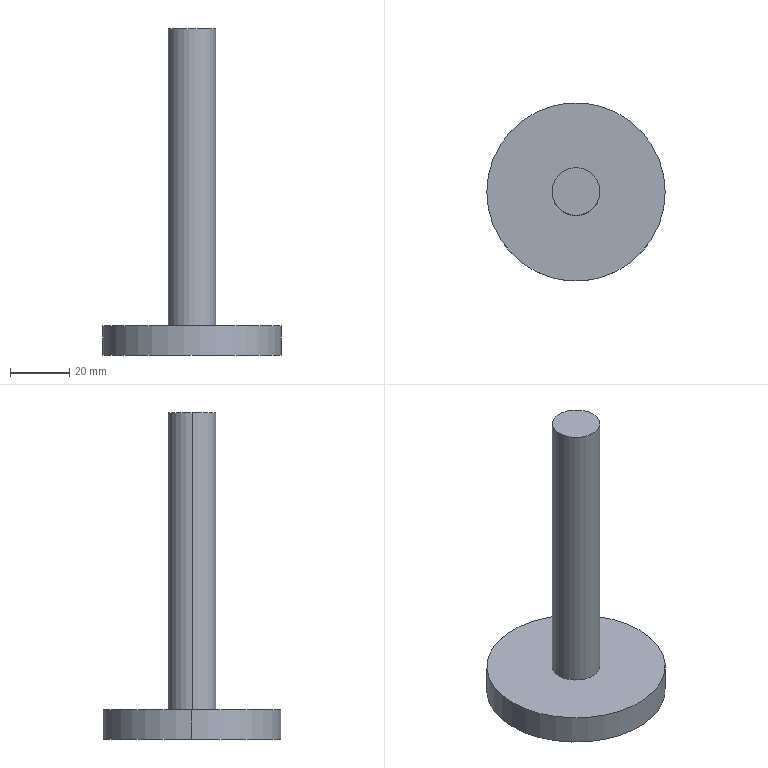Part | STEP file | CHAN TANGDUA | 1 solid | 7 faces | box 60 x 60 x 110 mm | volume 48381 mm3 | cylinder 4 | plane 3 | commonest cylinder face diameters 16 x2 60 x2
STEP:
#1=CARTESIAN_POINT('',(0.,0.,0.));
#2=DIRECTION('',(0.,0.,1.));
#3=DIRECTION('',(1.,0.,0.));
#4=AXIS2_PLACEMENT_3D('',#1,#2,#3);
#5=CARTESIAN_POINT('',(8.,0.,10.));
#6=VERTEX_POINT('',#5);
#7=CARTESIAN_POINT('',(-8.,0.,10.));
#8=VERTEX_POINT('',#7);
#9=CARTESIAN_POINT('',(0.,0.,10.));
#10=DIRECTION('',(0.,0.,1.));
#11=DIRECTION('',(1.,0.,0.));
#12=AXIS2_PLACEMENT_3D('',#9,#10,#11);
#13=CIRCLE('',#12,8.);
#14=CARTESIAN_POINT('',(0.,0.,10.));
#15=DIRECTION('',(0.,0.,1.));
#16=DIRECTION('',(1.,0.,0.));
#17=AXIS2_PLACEMENT_3D('',#14,#15,#16);
#18=CYLINDRICAL_SURFACE('',#17,8.);
#19=CARTESIAN_POINT('',(0.,0.));
#20=DIRECTION('',(1.,0.));
#21=VECTOR('',#20,1.);
#22=LINE('',#19,#21);
#23=(GEOMETRIC_REPRESENTATION_CONTEXT(2)PARAMETRIC_REPRESENTATION_CONTEXT()REPRESENTATION_CONTEXT('',''));
#24=DEFINITIONAL_REPRESENTATION('',(#22),#23);
#25=PCURVE('',#18,#24);
#26=CARTESIAN_POINT('',(0.,0.,10.));
#27=DIRECTION('',(0.,0.,-1.));
#28=DIRECTION('',(-1.,0.,0.));
#29=AXIS2_PLACEMENT_3D('',#26,#27,#28);
#30=PLANE('',#29);
#31=CARTESIAN_POINT('',(-8.,0.));
#32=CARTESIAN_POINT('',(-8.,13.856));
#33=CARTESIAN_POINT('',(4.,6.928));
#34=CARTESIAN_POINT('',(16.,0.));
#35=CARTESIAN_POINT('',(4.,-6.928));
#36=CARTESIAN_POINT('',(-8.,-13.856));
#37=CARTESIAN_POINT('',(-8.,0.));
#38=(BOUNDED_CURVE()B_SPLINE_CURVE(2,(#31,#32,#33,#34,#35,#36,#37),.UNSPECIFIED.,.T.,.F.)B_SPLINE_CURVE_WITH_KNOTS((1,2,2,2,2,1),(-2.094,0.,2.094,4.189,6.283,8.378),.UNSPECIFIED.)CURVE()GEOMETRIC_REPRESENTATION_ITEM()RATIONAL_B_SPLINE_CURVE((1.,0.5,1.,0.5,1.,0.5,1.))REPRESENTATION_ITEM(''));
#39=(GEOMETRIC_REPRESENTATION_CONTEXT(2)PARAMETRIC_REPRESENTATION_CONTEXT()REPRESENTATION_CONTEXT('',''));
#40=DEFINITIONAL_REPRESENTATION('',(#38),#39);
#41=PCURVE('',#30,#40);
#42=SURFACE_CURVE('',#13,(#25,#41),.PCURVE_S1.);
#43=EDGE_CURVE('',#6,#8,#42,.T.);
#44=ORIENTED_EDGE('',*,*,#43,.T.);
#45=CARTESIAN_POINT('',(-8.,0.,110.));
#46=VERTEX_POINT('',#45);
#47=CARTESIAN_POINT('',(-8.,0.,10.));
#48=DIRECTION('',(0.,0.,1.));
#49=VECTOR('',#48,1.);
#50=LINE('',#47,#49);
#51=CARTESIAN_POINT('',(3.142,0.));
#52=DIRECTION('',(0.,1.));
#53=VECTOR('',#52,1.);
#54=LINE('',#51,#53);
#55=(GEOMETRIC_REPRESENTATION_CONTEXT(2)PARAMETRIC_REPRESENTATION_CONTEXT()REPRESENTATION_CONTEXT('',''));
#56=DEFINITIONAL_REPRESENTATION('',(#54),#55);
#57=PCURVE('',#18,#56);
#58=CARTESIAN_POINT('',(0.,0.,10.));
#59=DIRECTION('',(0.,0.,1.));
#60=DIRECTION('',(1.,0.,0.));
#61=AXIS2_PLACEMENT_3D('',#58,#59,#60);
#62=CYLINDRICAL_SURFACE('',#61,8.);
#63=CARTESIAN_POINT('',(3.142,0.));
#64=DIRECTION('',(0.,1.));
#65=VECTOR('',#64,1.);
#66=LINE('',#63,#65);
#67=(GEOMETRIC_REPRESENTATION_CONTEXT(2)PARAMETRIC_REPRESENTATION_CONTEXT()REPRESENTATION_CONTEXT('',''));
#68=DEFINITIONAL_REPRESENTATION('',(#66),#67);
#69=PCURVE('',#62,#68);
#70=SURFACE_CURVE('',#50,(#57,#69),.PCURVE_S1.);
#71=EDGE_CURVE('',#8,#46,#70,.T.);
#72=ORIENTED_EDGE('',*,*,#71,.T.);
#73=CARTESIAN_POINT('',(8.,0.,110.));
#74=VERTEX_POINT('',#73);
#75=CARTESIAN_POINT('',(0.,0.,110.));
#76=DIRECTION('',(0.,0.,-1.));
#77=DIRECTION('',(1.,0.,0.));
#78=AXIS2_PLACEMENT_3D('',#75,#76,#77);
#79=CIRCLE('',#78,8.);
#80=CARTESIAN_POINT('',(6.283,100.));
#81=DIRECTION('',(-1.,0.));
#82=VECTOR('',#81,1.);
#83=LINE('',#80,#82);
#84=(GEOMETRIC_REPRESENTATION_CONTEXT(2)PARAMETRIC_REPRESENTATION_CONTEXT()REPRESENTATION_CONTEXT('',''));
#85=DEFINITIONAL_REPRESENTATION('',(#83),#84);
#86=PCURVE('',#18,#85);
#87=CARTESIAN_POINT('',(0.,0.,110.));
#88=DIRECTION('',(0.,0.,-1.));
#89=DIRECTION('',(-1.,0.,0.));
#90=AXIS2_PLACEMENT_3D('',#87,#88,#89);
#91=PLANE('',#90);
#92=CARTESIAN_POINT('',(0.,0.));
#93=DIRECTION('',(-1.,0.));
#94=AXIS2_PLACEMENT_2D('',#92,#93);
#95=CIRCLE('',#94,8.);
#96=(GEOMETRIC_REPRESENTATION_CONTEXT(2)PARAMETRIC_REPRESENTATION_CONTEXT()REPRESENTATION_CONTEXT('',''));
#97=DEFINITIONAL_REPRESENTATION('',(#95),#96);
#98=PCURVE('',#91,#97);
#99=SURFACE_CURVE('',#79,(#86,#98),.PCURVE_S1.);
#100=EDGE_CURVE('',#46,#74,#99,.T.);
#101=ORIENTED_EDGE('',*,*,#100,.T.);
#102=CARTESIAN_POINT('',(8.,0.,10.));
#103=DIRECTION('',(0.,0.,1.));
#104=VECTOR('',#103,1.);
#105=LINE('',#102,#104);
#106=CARTESIAN_POINT('',(0.,0.));
#107=DIRECTION('',(0.,1.));
#108=VECTOR('',#107,1.);
#109=LINE('',#106,#108);
#110=(GEOMETRIC_REPRESENTATION_CONTEXT(2)PARAMETRIC_REPRESENTATION_CONTEXT()REPRESENTATION_CONTEXT('',''));
#111=DEFINITIONAL_REPRESENTATION('',(#109),#110);
#112=PCURVE('',#18,#111);
#113=CARTESIAN_POINT('',(6.283,0.));
#114=DIRECTION('',(0.,1.));
#115=VECTOR('',#114,1.);
#116=LINE('',#113,#115);
#117=(GEOMETRIC_REPRESENTATION_CONTEXT(2)PARAMETRIC_REPRESENTATION_CONTEXT()REPRESENTATION_CONTEXT('',''));
#118=DEFINITIONAL_REPRESENTATION('',(#116),#117);
#119=PCURVE('',#62,#118);
#120=SURFACE_CURVE('',#105,(#112,#119),.PCURVE_S1.);
#121=EDGE_CURVE('',#6,#74,#120,.T.);
#122=ORIENTED_EDGE('',*,*,#121,.F.);
#123=EDGE_LOOP('',(#44,#72,#101,#122));
#124=FACE_BOUND('',#123,.T.);
#125=ADVANCED_FACE('',(#124),#18,.T.);
#126=CARTESIAN_POINT('',(30.,0.,0.));
#127=VERTEX_POINT('',#126);
#128=CARTESIAN_POINT('',(-30.,0.,0.));
#129=VERTEX_POINT('',#128);
#130=CARTESIAN_POINT('',(0.,0.,0.));
#131=DIRECTION('',(0.,0.,1.));
#132=DIRECTION('',(1.,0.,0.));
#133=AXIS2_PLACEMENT_3D('',#130,#131,#132);
#134=CIRCLE('',#133,30.);
#135=CARTESIAN_POINT('',(0.,0.,0.));
#136=DIRECTION('',(0.,0.,1.));
#137=DIRECTION('',(1.,0.,0.));
#138=AXIS2_PLACEMENT_3D('',#135,#136,#137);
#139=CYLINDRICAL_SURFACE('',#138,30.);
#140=CARTESIAN_POINT('',(0.,0.));
#141=DIRECTION('',(1.,0.));
#142=VECTOR('',#141,1.);
#143=LINE('',#140,#142);
#144=(GEOMETRIC_REPRESENTATION_CONTEXT(2)PARAMETRIC_REPRESENTATION_CONTEXT()REPRESENTATION_CONTEXT('',''));
#145=DEFINITIONAL_REPRESENTATION('',(#143),#144);
#146=PCURVE('',#139,#145);
#147=CARTESIAN_POINT('',(0.,0.,0.));
#148=DIRECTION('',(0.,0.,-1.));
#149=DIRECTION('',(-1.,0.,0.));
#150=AXIS2_PLACEMENT_3D('',#147,#148,#149);
#151=PLANE('',#150);
#152=CARTESIAN_POINT('',(-30.,0.));
#153=CARTESIAN_POINT('',(-30.,51.962));
#154=CARTESIAN_POINT('',(15.,25.981));
#155=CARTESIAN_POINT('',(60.,0.));
#156=CARTESIAN_POINT('',(15.,-25.981));
#157=CARTESIAN_POINT('',(-30.,-51.962));
#158=CARTESIAN_POINT('',(-30.,0.));
#159=(BOUNDED_CURVE()B_SPLINE_CURVE(2,(#152,#153,#154,#155,#156,#157,#158),.UNSPECIFIED.,.T.,.F.)B_SPLINE_CURVE_WITH_KNOTS((1,2,2,2,2,1),(-2.094,0.,2.094,4.189,6.283,8.378),.UNSPECIFIED.)CURVE()GEOMETRIC_REPRESENTATION_ITEM()RATIONAL_B_SPLINE_CURVE((1.,0.5,1.,0.5,1.,0.5,1.))REPRESENTATION_ITEM(''));
#160=(GEOMETRIC_REPRESENTATION_CONTEXT(2)PARAMETRIC_REPRESENTATION_CONTEXT()REPRESENTATION_CONTEXT('',''));
#161=DEFINITIONAL_REPRESENTATION('',(#159),#160);
#162=PCURVE('',#151,#161);
#163=SURFACE_CURVE('',#134,(#146,#162),.PCURVE_S1.);
#164=EDGE_CURVE('',#127,#129,#163,.T.);
#165=ORIENTED_EDGE('',*,*,#164,.T.);
#166=CARTESIAN_POINT('',(-30.,0.,10.));
#167=VERTEX_POINT('',#166);
#168=CARTESIAN_POINT('',(-30.,0.,0.));
#169=DIRECTION('',(0.,0.,1.));
#170=VECTOR('',#169,1.);
#171=LINE('',#168,#170);
#172=CARTESIAN_POINT('',(3.142,0.));
#173=DIRECTION('',(0.,1.));
#174=VECTOR('',#173,1.);
#175=LINE('',#172,#174);
#176=(GEOMETRIC_REPRESENTATION_CONTEXT(2)PARAMETRIC_REPRESENTATION_CONTEXT()REPRESENTATION_CONTEXT('',''));
#177=DEFINITIONAL_REPRESENTATION('',(#175),#176);
#178=PCURVE('',#139,#177);
#179=CARTESIAN_POINT('',(0.,0.,0.));
#180=DIRECTION('',(0.,0.,1.));
#181=DIRECTION('',(1.,0.,0.));
#182=AXIS2_PLACEMENT_3D('',#179,#180,#181);
#183=CYLINDRICAL_SURFACE('',#182,30.);
#184=CARTESIAN_POINT('',(3.142,0.));
#185=DIRECTION('',(0.,1.));
#186=VECTOR('',#185,1.);
#187=LINE('',#184,#186);
#188=(GEOMETRIC_REPRESENTATION_CONTEXT(2)PARAMETRIC_REPRESENTATION_CONTEXT()REPRESENTATION_CONTEXT('',''));
#189=DEFINITIONAL_REPRESENTATION('',(#187),#188);
#190=PCURVE('',#183,#189);
#191=SURFACE_CURVE('',#171,(#178,#190),.PCURVE_S1.);
#192=EDGE_CURVE('',#129,#167,#191,.T.);
#193=ORIENTED_EDGE('',*,*,#192,.T.);
#194=CARTESIAN_POINT('',(30.,0.,10.));
#195=VERTEX_POINT('',#194);
#196=CARTESIAN_POINT('',(0.,0.,10.));
#197=DIRECTION('',(0.,0.,-1.));
#198=DIRECTION('',(1.,0.,0.));
#199=AXIS2_PLACEMENT_3D('',#196,#197,#198);
#200=CIRCLE('',#199,30.);
#201=CARTESIAN_POINT('',(6.283,10.));
#202=DIRECTION('',(-1.,0.));
#203=VECTOR('',#202,1.);
#204=LINE('',#201,#203);
#205=(GEOMETRIC_REPRESENTATION_CONTEXT(2)PARAMETRIC_REPRESENTATION_CONTEXT()REPRESENTATION_CONTEXT('',''));
#206=DEFINITIONAL_REPRESENTATION('',(#204),#205);
#207=PCURVE('',#139,#206);
#208=CARTESIAN_POINT('',(0.,0.));
#209=DIRECTION('',(-1.,0.));
#210=AXIS2_PLACEMENT_2D('',#208,#209);
#211=CIRCLE('',#210,30.);
#212=(GEOMETRIC_REPRESENTATION_CONTEXT(2)PARAMETRIC_REPRESENTATION_CONTEXT()REPRESENTATION_CONTEXT('',''));
#213=DEFINITIONAL_REPRESENTATION('',(#211),#212);
#214=PCURVE('',#30,#213);
#215=SURFACE_CURVE('',#200,(#207,#214),.PCURVE_S1.);
#216=EDGE_CURVE('',#167,#195,#215,.T.);
#217=ORIENTED_EDGE('',*,*,#216,.T.);
#218=CARTESIAN_POINT('',(30.,0.,0.));
#219=DIRECTION('',(0.,0.,1.));
#220=VECTOR('',#219,1.);
#221=LINE('',#218,#220);
#222=CARTESIAN_POINT('',(0.,0.));
#223=DIRECTION('',(0.,1.));
#224=VECTOR('',#223,1.);
#225=LINE('',#222,#224);
#226=(GEOMETRIC_REPRESENTATION_CONTEXT(2)PARAMETRIC_REPRESENTATION_CONTEXT()REPRESENTATION_CONTEXT('',''));
#227=DEFINITIONAL_REPRESENTATION('',(#225),#226);
#228=PCURVE('',#139,#227);
#229=CARTESIAN_POINT('',(6.283,0.));
#230=DIRECTION('',(0.,1.));
#231=VECTOR('',#230,1.);
#232=LINE('',#229,#231);
#233=(GEOMETRIC_REPRESENTATION_CONTEXT(2)PARAMETRIC_REPRESENTATION_CONTEXT()REPRESENTATION_CONTEXT('',''));
#234=DEFINITIONAL_REPRESENTATION('',(#232),#233);
#235=PCURVE('',#183,#234);
#236=SURFACE_CURVE('',#221,(#228,#235),.PCURVE_S1.);
#237=EDGE_CURVE('',#127,#195,#236,.T.);
#238=ORIENTED_EDGE('',*,*,#237,.F.);
#239=EDGE_LOOP('',(#165,#193,#217,#238));
#240=FACE_BOUND('',#239,.T.);
#241=ADVANCED_FACE('',(#240),#139,.T.);
#242=ORIENTED_EDGE('',*,*,#71,.F.);
#243=CARTESIAN_POINT('',(0.,0.,10.));
#244=DIRECTION('',(0.,0.,1.));
#245=DIRECTION('',(1.,0.,0.));
#246=AXIS2_PLACEMENT_3D('',#243,#244,#245);
#247=CIRCLE('',#246,8.);
#248=CARTESIAN_POINT('',(0.,0.));
#249=DIRECTION('',(1.,0.));
#250=VECTOR('',#249,1.);
#251=LINE('',#248,#250);
#252=(GEOMETRIC_REPRESENTATION_CONTEXT(2)PARAMETRIC_REPRESENTATION_CONTEXT()REPRESENTATION_CONTEXT('',''));
#253=DEFINITIONAL_REPRESENTATION('',(#251),#252);
#254=PCURVE('',#62,#253);
#255=CARTESIAN_POINT('',(-8.,0.));
#256=CARTESIAN_POINT('',(-8.,13.856));
#257=CARTESIAN_POINT('',(4.,6.928));
#258=CARTESIAN_POINT('',(16.,0.));
#259=CARTESIAN_POINT('',(4.,-6.928));
#260=CARTESIAN_POINT('',(-8.,-13.856));
#261=CARTESIAN_POINT('',(-8.,0.));
#262=(BOUNDED_CURVE()B_SPLINE_CURVE(2,(#255,#256,#257,#258,#259,#260,#261),.UNSPECIFIED.,.T.,.F.)B_SPLINE_CURVE_WITH_KNOTS((1,2,2,2,2,1),(-2.094,0.,2.094,4.189,6.283,8.378),.UNSPECIFIED.)CURVE()GEOMETRIC_REPRESENTATION_ITEM()RATIONAL_B_SPLINE_CURVE((1.,0.5,1.,0.5,1.,0.5,1.))REPRESENTATION_ITEM(''));
#263=(GEOMETRIC_REPRESENTATION_CONTEXT(2)PARAMETRIC_REPRESENTATION_CONTEXT()REPRESENTATION_CONTEXT('',''));
#264=DEFINITIONAL_REPRESENTATION('',(#262),#263);
#265=PCURVE('',#30,#264);
#266=SURFACE_CURVE('',#247,(#254,#265),.PCURVE_S1.);
#267=EDGE_CURVE('',#8,#6,#266,.T.);
#268=ORIENTED_EDGE('',*,*,#267,.T.);
#269=ORIENTED_EDGE('',*,*,#121,.T.);
#270=CARTESIAN_POINT('',(0.,0.,110.));
#271=DIRECTION('',(0.,0.,-1.));
#272=DIRECTION('',(1.,0.,0.));
#273=AXIS2_PLACEMENT_3D('',#270,#271,#272);
#274=CIRCLE('',#273,8.);
#275=CARTESIAN_POINT('',(6.283,100.));
#276=DIRECTION('',(-1.,0.));
#277=VECTOR('',#276,1.);
#278=LINE('',#275,#277);
#279=(GEOMETRIC_REPRESENTATION_CONTEXT(2)PARAMETRIC_REPRESENTATION_CONTEXT()REPRESENTATION_CONTEXT('',''));
#280=DEFINITIONAL_REPRESENTATION('',(#278),#279);
#281=PCURVE('',#62,#280);
#282=CARTESIAN_POINT('',(0.,0.));
#283=DIRECTION('',(-1.,0.));
#284=AXIS2_PLACEMENT_2D('',#282,#283);
#285=CIRCLE('',#284,8.);
#286=(GEOMETRIC_REPRESENTATION_CONTEXT(2)PARAMETRIC_REPRESENTATION_CONTEXT()REPRESENTATION_CONTEXT('',''));
#287=DEFINITIONAL_REPRESENTATION('',(#285),#286);
#288=PCURVE('',#91,#287);
#289=SURFACE_CURVE('',#274,(#281,#288),.PCURVE_S1.);
#290=EDGE_CURVE('',#74,#46,#289,.T.);
#291=ORIENTED_EDGE('',*,*,#290,.T.);
#292=EDGE_LOOP('',(#242,#268,#269,#291));
#293=FACE_BOUND('',#292,.T.);
#294=ADVANCED_FACE('',(#293),#62,.T.);
#295=ORIENTED_EDGE('',*,*,#43,.F.);
#296=ORIENTED_EDGE('',*,*,#267,.F.);
#297=EDGE_LOOP('',(#295,#296));
#298=FACE_BOUND('',#297,.T.);
#299=CARTESIAN_POINT('',(0.,0.,10.));
#300=DIRECTION('',(0.,0.,-1.));
#301=DIRECTION('',(1.,0.,0.));
#302=AXIS2_PLACEMENT_3D('',#299,#300,#301);
#303=CIRCLE('',#302,30.);
#304=CARTESIAN_POINT('',(0.,0.));
#305=DIRECTION('',(-1.,0.));
#306=AXIS2_PLACEMENT_2D('',#304,#305);
#307=CIRCLE('',#306,30.);
#308=(GEOMETRIC_REPRESENTATION_CONTEXT(2)PARAMETRIC_REPRESENTATION_CONTEXT()REPRESENTATION_CONTEXT('',''));
#309=DEFINITIONAL_REPRESENTATION('',(#307),#308);
#310=PCURVE('',#30,#309);
#311=CARTESIAN_POINT('',(6.283,10.));
#312=DIRECTION('',(-1.,0.));
#313=VECTOR('',#312,1.);
#314=LINE('',#311,#313);
#315=(GEOMETRIC_REPRESENTATION_CONTEXT(2)PARAMETRIC_REPRESENTATION_CONTEXT()REPRESENTATION_CONTEXT('',''));
#316=DEFINITIONAL_REPRESENTATION('',(#314),#315);
#317=PCURVE('',#183,#316);
#318=SURFACE_CURVE('',#303,(#310,#317),.PCURVE_S1.);
#319=EDGE_CURVE('',#195,#167,#318,.T.);
#320=ORIENTED_EDGE('',*,*,#319,.F.);
#321=ORIENTED_EDGE('',*,*,#216,.F.);
#322=EDGE_LOOP('',(#320,#321));
#323=FACE_BOUND('',#322,.T.);
#324=ADVANCED_FACE('',(#298,#323),#30,.F.);
#325=ORIENTED_EDGE('',*,*,#290,.F.);
#326=ORIENTED_EDGE('',*,*,#100,.F.);
#327=EDGE_LOOP('',(#325,#326));
#328=FACE_BOUND('',#327,.T.);
#329=ADVANCED_FACE('',(#328),#91,.F.);
#330=ORIENTED_EDGE('',*,*,#192,.F.);
#331=CARTESIAN_POINT('',(0.,0.,0.));
#332=DIRECTION('',(0.,0.,1.));
#333=DIRECTION('',(1.,0.,0.));
#334=AXIS2_PLACEMENT_3D('',#331,#332,#333);
#335=CIRCLE('',#334,30.);
#336=CARTESIAN_POINT('',(0.,0.));
#337=DIRECTION('',(1.,0.));
#338=VECTOR('',#337,1.);
#339=LINE('',#336,#338);
#340=(GEOMETRIC_REPRESENTATION_CONTEXT(2)PARAMETRIC_REPRESENTATION_CONTEXT()REPRESENTATION_CONTEXT('',''));
#341=DEFINITIONAL_REPRESENTATION('',(#339),#340);
#342=PCURVE('',#183,#341);
#343=CARTESIAN_POINT('',(-30.,0.));
#344=CARTESIAN_POINT('',(-30.,51.962));
#345=CARTESIAN_POINT('',(15.,25.981));
#346=CARTESIAN_POINT('',(60.,0.));
#347=CARTESIAN_POINT('',(15.,-25.981));
#348=CARTESIAN_POINT('',(-30.,-51.962));
#349=CARTESIAN_POINT('',(-30.,0.));
#350=(BOUNDED_CURVE()B_SPLINE_CURVE(2,(#343,#344,#345,#346,#347,#348,#349),.UNSPECIFIED.,.T.,.F.)B_SPLINE_CURVE_WITH_KNOTS((1,2,2,2,2,1),(-2.094,0.,2.094,4.189,6.283,8.378),.UNSPECIFIED.)CURVE()GEOMETRIC_REPRESENTATION_ITEM()RATIONAL_B_SPLINE_CURVE((1.,0.5,1.,0.5,1.,0.5,1.))REPRESENTATION_ITEM(''));
#351=(GEOMETRIC_REPRESENTATION_CONTEXT(2)PARAMETRIC_REPRESENTATION_CONTEXT()REPRESENTATION_CONTEXT('',''));
#352=DEFINITIONAL_REPRESENTATION('',(#350),#351);
#353=PCURVE('',#151,#352);
#354=SURFACE_CURVE('',#335,(#342,#353),.PCURVE_S1.);
#355=EDGE_CURVE('',#129,#127,#354,.T.);
#356=ORIENTED_EDGE('',*,*,#355,.T.);
#357=ORIENTED_EDGE('',*,*,#237,.T.);
#358=ORIENTED_EDGE('',*,*,#319,.T.);
#359=EDGE_LOOP('',(#330,#356,#357,#358));
#360=FACE_BOUND('',#359,.T.);
#361=ADVANCED_FACE('',(#360),#183,.T.);
#362=ORIENTED_EDGE('',*,*,#164,.F.);
#363=ORIENTED_EDGE('',*,*,#355,.F.);
#364=EDGE_LOOP('',(#362,#363));
#365=FACE_BOUND('',#364,.T.);
#366=ADVANCED_FACE('',(#365),#151,.T.);
#367=CLOSED_SHELL('',(#125,#241,#294,#324,#329,#361,#366));
#368=MANIFOLD_SOLID_BREP('',#367);
#369=(LENGTH_UNIT()NAMED_UNIT(*)SI_UNIT(.MILLI.,.METRE.));
#370=UNCERTAINTY_MEASURE_WITH_UNIT(LENGTH_MEASURE(0.0000001),#369,'','');
#371=(NAMED_UNIT(*)PLANE_ANGLE_UNIT()SI_UNIT($,.RADIAN.));
#372=(NAMED_UNIT(*)SI_UNIT($,.STERADIAN.)SOLID_ANGLE_UNIT());
#373=(GEOMETRIC_REPRESENTATION_CONTEXT(3)GLOBAL_UNCERTAINTY_ASSIGNED_CONTEXT((#370))GLOBAL_UNIT_ASSIGNED_CONTEXT((#369,#371,#372))REPRESENTATION_CONTEXT('',''));
#374=ADVANCED_BREP_SHAPE_REPRESENTATION('',(#4,#368),#373);